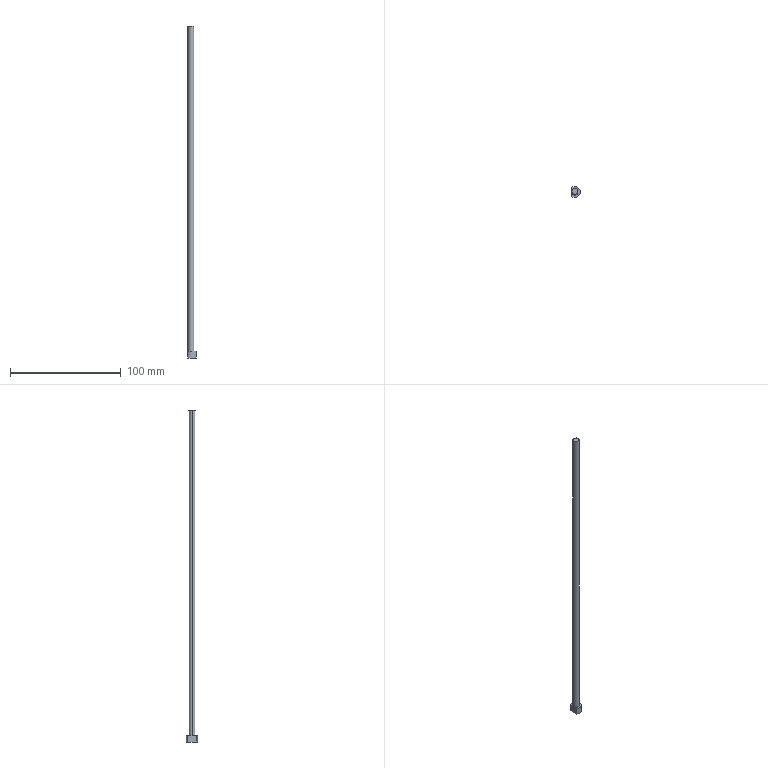Part | Creo | 1 solid | 7 faces | box 8 x 10 x 299.128 mm | volume 7368 mm3 | plane 4 | cylinder 3 | commonest cylinder face diameters 5.5 x2 10 x1
STEP:
#1=CARTESIAN_POINT('',(-86.,17.,-296.));
#2=VERTEX_POINT('',#1);
#3=CARTESIAN_POINT('',(-86.,9.,-296.));
#4=VERTEX_POINT('',#3);
#5=CARTESIAN_POINT('',(-83.,13.,-296.));
#6=DIRECTION('',(0.,0.,-1.));
#7=DIRECTION('',(-0.6,0.8,0.));
#8=AXIS2_PLACEMENT_3D('',#5,#6,#7);
#9=CIRCLE('',#8,5.);
#10=EDGE_CURVE('',#2,#4,#9,.T.);
#11=ORIENTED_EDGE('',*,*,#10,.F.);
#12=CARTESIAN_POINT('',(-86.,17.,-296.));
#13=DIRECTION('',(0.,-1.,0.));
#14=VECTOR('',#13,8.);
#15=LINE('',#12,#14);
#16=EDGE_CURVE('',#2,#4,#15,.T.);
#17=ORIENTED_EDGE('',*,*,#16,.T.);
#18=EDGE_LOOP('',(#11,#17));
#19=FACE_OUTER_BOUND('',#18,.F.);
#20=CARTESIAN_POINT('',(10.,-0.004699,-296.));
#21=DIRECTION('',(0.,0.,1.));
#22=DIRECTION('',(0.,1.,0.));
#23=AXIS2_PLACEMENT_3D('',#20,#21,#22);
#24=PLANE('',#23);
#25=ADVANCED_FACE('',(#19),#24,.F.);
#26=CARTESIAN_POINT('',(-86.,17.,-290.));
#27=VERTEX_POINT('',#26);
#28=CARTESIAN_POINT('',(-86.,17.,-296.));
#29=DIRECTION('',(0.,0.,1.));
#30=VECTOR('',#29,6.);
#31=LINE('',#28,#30);
#32=EDGE_CURVE('',#2,#27,#31,.T.);
#33=ORIENTED_EDGE('',*,*,#32,.F.);
#34=ORIENTED_EDGE('',*,*,#10,.T.);
#35=CARTESIAN_POINT('',(-86.,9.,-290.));
#36=VERTEX_POINT('',#35);
#37=CARTESIAN_POINT('',(-86.,9.,-290.));
#38=DIRECTION('',(0.,0.,-1.));
#39=VECTOR('',#38,6.);
#40=LINE('',#37,#39);
#41=EDGE_CURVE('',#36,#4,#40,.T.);
#42=ORIENTED_EDGE('',*,*,#41,.F.);
#43=CARTESIAN_POINT('',(-83.,13.,-290.));
#44=DIRECTION('',(0.,0.,1.));
#45=DIRECTION('',(-0.6,-0.8,0.));
#46=AXIS2_PLACEMENT_3D('',#43,#44,#45);
#47=CIRCLE('',#46,5.);
#48=EDGE_CURVE('',#36,#27,#47,.T.);
#49=ORIENTED_EDGE('',*,*,#48,.T.);
#50=EDGE_LOOP('',(#33,#34,#42,#49));
#51=FACE_OUTER_BOUND('',#50,.F.);
#52=CARTESIAN_POINT('',(-83.,13.,-296.));
#53=DIRECTION('',(0.,0.,1.));
#54=DIRECTION('',(-1.,0.,0.));
#55=AXIS2_PLACEMENT_3D('',#52,#53,#54);
#56=CYLINDRICAL_SURFACE('',#55,5.);
#57=ADVANCED_FACE('',(#51),#56,.T.);
#58=ORIENTED_EDGE('',*,*,#32,.T.);
#59=CARTESIAN_POINT('',(-86.,17.,-290.));
#60=DIRECTION('',(0.,-1.,0.));
#61=VECTOR('',#60,8.);
#62=LINE('',#59,#61);
#63=EDGE_CURVE('',#27,#36,#62,.T.);
#64=ORIENTED_EDGE('',*,*,#63,.T.);
#65=ORIENTED_EDGE('',*,*,#41,.T.);
#66=ORIENTED_EDGE('',*,*,#16,.F.);
#67=EDGE_LOOP('',(#58,#64,#65,#66));
#68=FACE_OUTER_BOUND('',#67,.F.);
#69=CARTESIAN_POINT('',(-86.,13.,-296.));
#70=DIRECTION('',(1.,0.,0.));
#71=DIRECTION('',(0.,0.,1.));
#72=AXIS2_PLACEMENT_3D('',#69,#70,#71);
#73=PLANE('',#72);
#74=ADVANCED_FACE('',(#68),#73,.F.);
#75=ORIENTED_EDGE('',*,*,#63,.F.);
#76=ORIENTED_EDGE('',*,*,#48,.F.);
#77=EDGE_LOOP('',(#75,#76));
#78=FACE_OUTER_BOUND('',#77,.F.);
#79=CARTESIAN_POINT('',(-80.25,13.,-290.));
#80=VERTEX_POINT('',#79);
#81=CARTESIAN_POINT('',(-85.75,13.,-290.));
#82=VERTEX_POINT('',#81);
#83=CARTESIAN_POINT('',(-83.,13.,-290.));
#84=DIRECTION('',(0.,0.,-1.));
#85=DIRECTION('',(1.,0.,0.));
#86=AXIS2_PLACEMENT_3D('',#83,#84,#85);
#87=CIRCLE('',#86,2.75);
#88=EDGE_CURVE('',#80,#82,#87,.T.);
#89=ORIENTED_EDGE('',*,*,#88,.F.);
#90=CARTESIAN_POINT('',(-83.,13.,-290.));
#91=DIRECTION('',(0.,0.,-1.));
#92=DIRECTION('',(-1.,0.,0.));
#93=AXIS2_PLACEMENT_3D('',#90,#91,#92);
#94=CIRCLE('',#93,2.75);
#95=EDGE_CURVE('',#82,#80,#94,.T.);
#96=ORIENTED_EDGE('',*,*,#95,.F.);
#97=EDGE_LOOP('',(#89,#96));
#98=FACE_BOUND('',#97,.F.);
#99=CARTESIAN_POINT('',(-83.,13.,-290.));
#100=DIRECTION('',(0.,0.,1.));
#101=DIRECTION('',(-1.,0.,0.));
#102=AXIS2_PLACEMENT_3D('',#99,#100,#101);
#103=PLANE('',#102);
#104=ADVANCED_FACE('',(#78,#98),#103,.T.);
#105=ORIENTED_EDGE('',*,*,#88,.T.);
#106=CARTESIAN_POINT('',(-85.75,13.,3.128));
#107=VERTEX_POINT('',#106);
#108=CARTESIAN_POINT('',(-85.75,13.,3.128));
#109=DIRECTION('',(0.,0.,-1.));
#110=VECTOR('',#109,293.128);
#111=LINE('',#108,#110);
#112=EDGE_CURVE('',#107,#82,#111,.T.);
#113=ORIENTED_EDGE('',*,*,#112,.F.);
#114=CARTESIAN_POINT('',(-80.25,13.,3.128));
#115=VERTEX_POINT('',#114);
#116=CARTESIAN_POINT('',(-83.,13.,3.128));
#117=DIRECTION('',(0.,0.,1.));
#118=DIRECTION('',(-1.,0.,0.));
#119=AXIS2_PLACEMENT_3D('',#116,#117,#118);
#120=CIRCLE('',#119,2.75);
#121=EDGE_CURVE('',#107,#115,#120,.T.);
#122=ORIENTED_EDGE('',*,*,#121,.T.);
#123=CARTESIAN_POINT('',(-80.25,13.,3.128));
#124=DIRECTION('',(0.,0.,-1.));
#125=VECTOR('',#124,293.128);
#126=LINE('',#123,#125);
#127=EDGE_CURVE('',#115,#80,#126,.T.);
#128=ORIENTED_EDGE('',*,*,#127,.T.);
#129=EDGE_LOOP('',(#105,#113,#122,#128));
#130=FACE_OUTER_BOUND('',#129,.F.);
#131=CARTESIAN_POINT('',(-83.,13.,95.));
#132=DIRECTION('',(0.,0.,-1.));
#133=DIRECTION('',(1.,0.,0.));
#134=AXIS2_PLACEMENT_3D('',#131,#132,#133);
#135=CYLINDRICAL_SURFACE('',#134,2.75);
#136=ADVANCED_FACE('',(#130),#135,.T.);
#137=ORIENTED_EDGE('',*,*,#95,.T.);
#138=ORIENTED_EDGE('',*,*,#127,.F.);
#139=CARTESIAN_POINT('',(-83.,13.,3.128));
#140=DIRECTION('',(0.,0.,1.));
#141=DIRECTION('',(1.,0.,0.));
#142=AXIS2_PLACEMENT_3D('',#139,#140,#141);
#143=CIRCLE('',#142,2.75);
#144=EDGE_CURVE('',#115,#107,#143,.T.);
#145=ORIENTED_EDGE('',*,*,#144,.T.);
#146=ORIENTED_EDGE('',*,*,#112,.T.);
#147=EDGE_LOOP('',(#137,#138,#145,#146));
#148=FACE_OUTER_BOUND('',#147,.F.);
#149=CARTESIAN_POINT('',(-83.,13.,95.));
#150=DIRECTION('',(0.,0.,-1.));
#151=DIRECTION('',(1.,0.,0.));
#152=AXIS2_PLACEMENT_3D('',#149,#150,#151);
#153=CYLINDRICAL_SURFACE('',#152,2.75);
#154=ADVANCED_FACE('',(#148),#153,.T.);
#155=ORIENTED_EDGE('',*,*,#144,.F.);
#156=ORIENTED_EDGE('',*,*,#121,.F.);
#157=EDGE_LOOP('',(#155,#156));
#158=FACE_OUTER_BOUND('',#157,.F.);
#159=CARTESIAN_POINT('',(0.,0.,3.128));
#160=DIRECTION('',(0.,0.,1.));
#161=DIRECTION('',(0.,1.,0.));
#162=AXIS2_PLACEMENT_3D('',#159,#160,#161);
#163=PLANE('',#162);
#164=ADVANCED_FACE('',(#158),#163,.T.);
#165=CLOSED_SHELL('',(#25,#57,#74,#104,#136,#154,#164));
#166=MANIFOLD_SOLID_BREP('',#165);
#167=(LENGTH_UNIT()NAMED_UNIT(*)SI_UNIT(.MILLI.,.METRE.));
#168=UNCERTAINTY_MEASURE_WITH_UNIT(LENGTH_MEASURE(0.02994),#167,'','');
#169=(NAMED_UNIT(*)PLANE_ANGLE_UNIT()SI_UNIT($,.RADIAN.));
#170=PLANE_ANGLE_MEASURE_WITH_UNIT(PLANE_ANGLE_MEASURE(0.01745),#169);
#171=(CONVERSION_BASED_UNIT('DEGREE',#170)NAMED_UNIT(*)PLANE_ANGLE_UNIT());
#172=(NAMED_UNIT(*)SI_UNIT($,.STERADIAN.)SOLID_ANGLE_UNIT());
#173=(GEOMETRIC_REPRESENTATION_CONTEXT(3)GLOBAL_UNCERTAINTY_ASSIGNED_CONTEXT((#168))GLOBAL_UNIT_ASSIGNED_CONTEXT((#167,#171,#172))REPRESENTATION_CONTEXT('',''));
#174=ADVANCED_BREP_SHAPE_REPRESENTATION('',(#166),#173);